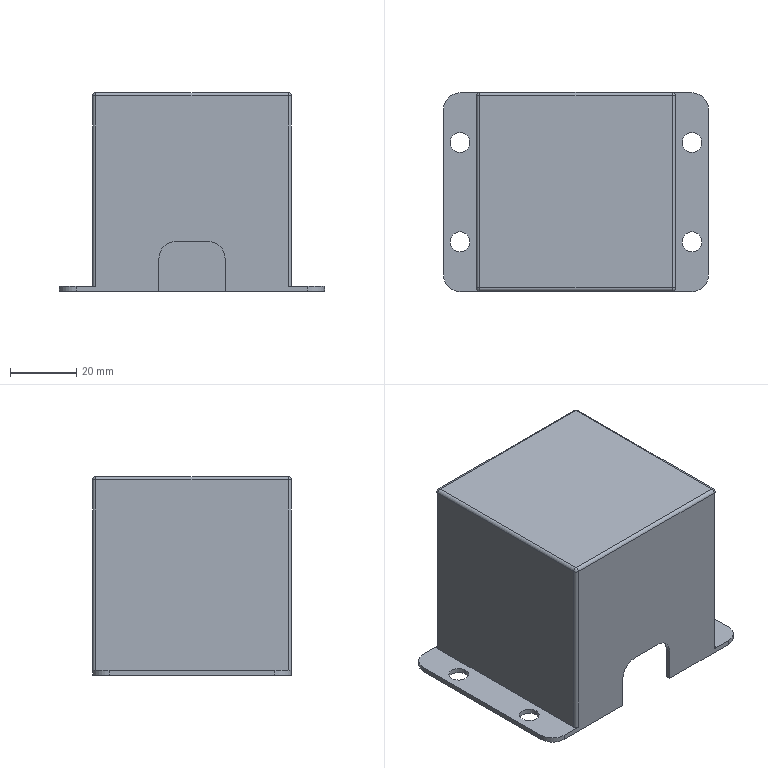Part | SolidWorks | features ICE 4, Fillet 3, Cut 1, Extrusion 1, MirrorPattern 1, Shell 1 | 1 solid | 46 faces | box 80 x 60 x 60 mm | volume 26373 mm3 | cylinder 24 | plane 18 | sphere 4 | commonest cylinder face diameters 2 x8 6 x8 10 x6 23 x2
STEP:
#1=CARTESIAN_POINT('',(-32.,15.,-30.));
#2=VERTEX_POINT('',#1);
#3=CARTESIAN_POINT('',(-38.,15.,-30.));
#4=VERTEX_POINT('',#3);
#5=CARTESIAN_POINT('',(-35.,15.,-30.));
#6=DIRECTION('',(0.,0.,-1.));
#7=DIRECTION('',(-1.,0.,0.));
#8=AXIS2_PLACEMENT_3D('',#5,#6,#7);
#9=CIRCLE('',#8,3.);
#10=EDGE_CURVE('',#2,#4,#9,.T.);
#11=ORIENTED_EDGE('',*,*,#10,.T.);
#12=CARTESIAN_POINT('',(-38.,15.,-28.5));
#13=VERTEX_POINT('',#12);
#14=CARTESIAN_POINT('',(-38.,15.,-30.));
#15=DIRECTION('',(0.,0.,1.));
#16=VECTOR('',#15,1000.);
#17=LINE('',#14,#16);
#18=EDGE_CURVE('',#4,#13,#17,.T.);
#19=ORIENTED_EDGE('',*,*,#18,.T.);
#20=CARTESIAN_POINT('',(-32.,15.,-28.5));
#21=VERTEX_POINT('',#20);
#22=CARTESIAN_POINT('',(-35.,15.,-28.5));
#23=DIRECTION('',(0.,0.,-1.));
#24=DIRECTION('',(-1.,0.,0.));
#25=AXIS2_PLACEMENT_3D('',#22,#23,#24);
#26=CIRCLE('',#25,3.);
#27=EDGE_CURVE('',#21,#13,#26,.T.);
#28=ORIENTED_EDGE('',*,*,#27,.F.);
#29=CARTESIAN_POINT('',(-32.,15.,-30.));
#30=DIRECTION('',(0.,0.,1.));
#31=VECTOR('',#30,1000.);
#32=LINE('',#29,#31);
#33=EDGE_CURVE('',#2,#21,#32,.T.);
#34=ORIENTED_EDGE('',*,*,#33,.F.);
#35=EDGE_LOOP('',(#11,#19,#28,#34));
#36=FACE_OUTER_BOUND('',#35,.T.);
#37=CARTESIAN_POINT('',(-35.,15.,-30.));
#38=DIRECTION('',(0.,0.,1.));
#39=DIRECTION('',(1.,0.,0.));
#40=AXIS2_PLACEMENT_3D('',#37,#38,#39);
#41=CYLINDRICAL_SURFACE('',#40,3.);
#42=ADVANCED_FACE('',(#36),#41,.F.);
#43=CARTESIAN_POINT('',(-32.,-15.,-30.));
#44=VERTEX_POINT('',#43);
#45=CARTESIAN_POINT('',(-38.,-15.,-30.));
#46=VERTEX_POINT('',#45);
#47=CARTESIAN_POINT('',(-35.,-15.,-30.));
#48=DIRECTION('',(0.,0.,-1.));
#49=DIRECTION('',(-1.,0.,0.));
#50=AXIS2_PLACEMENT_3D('',#47,#48,#49);
#51=CIRCLE('',#50,3.);
#52=EDGE_CURVE('',#44,#46,#51,.T.);
#53=ORIENTED_EDGE('',*,*,#52,.T.);
#54=CARTESIAN_POINT('',(-38.,-15.,-28.5));
#55=VERTEX_POINT('',#54);
#56=CARTESIAN_POINT('',(-38.,-15.,-30.));
#57=DIRECTION('',(0.,0.,1.));
#58=VECTOR('',#57,1000.);
#59=LINE('',#56,#58);
#60=EDGE_CURVE('',#46,#55,#59,.T.);
#61=ORIENTED_EDGE('',*,*,#60,.T.);
#62=CARTESIAN_POINT('',(-32.,-15.,-28.5));
#63=VERTEX_POINT('',#62);
#64=CARTESIAN_POINT('',(-35.,-15.,-28.5));
#65=DIRECTION('',(0.,0.,-1.));
#66=DIRECTION('',(-1.,0.,0.));
#67=AXIS2_PLACEMENT_3D('',#64,#65,#66);
#68=CIRCLE('',#67,3.);
#69=EDGE_CURVE('',#63,#55,#68,.T.);
#70=ORIENTED_EDGE('',*,*,#69,.F.);
#71=CARTESIAN_POINT('',(-32.,-15.,-30.));
#72=DIRECTION('',(0.,0.,1.));
#73=VECTOR('',#72,1000.);
#74=LINE('',#71,#73);
#75=EDGE_CURVE('',#44,#63,#74,.T.);
#76=ORIENTED_EDGE('',*,*,#75,.F.);
#77=EDGE_LOOP('',(#53,#61,#70,#76));
#78=FACE_OUTER_BOUND('',#77,.T.);
#79=CARTESIAN_POINT('',(-35.,-15.,-30.));
#80=DIRECTION('',(0.,0.,1.));
#81=DIRECTION('',(1.,0.,0.));
#82=AXIS2_PLACEMENT_3D('',#79,#80,#81);
#83=CYLINDRICAL_SURFACE('',#82,3.);
#84=ADVANCED_FACE('',(#78),#83,.F.);
#85=CARTESIAN_POINT('',(32.,15.,-30.));
#86=VERTEX_POINT('',#85);
#87=CARTESIAN_POINT('',(38.,15.,-30.));
#88=VERTEX_POINT('',#87);
#89=CARTESIAN_POINT('',(35.,15.,-30.));
#90=DIRECTION('',(0.,0.,1.));
#91=DIRECTION('',(1.,0.,0.));
#92=AXIS2_PLACEMENT_3D('',#89,#90,#91);
#93=CIRCLE('',#92,3.);
#94=EDGE_CURVE('',#86,#88,#93,.T.);
#95=ORIENTED_EDGE('',*,*,#94,.F.);
#96=CARTESIAN_POINT('',(32.,15.,-28.5));
#97=VERTEX_POINT('',#96);
#98=CARTESIAN_POINT('',(32.,15.,-30.));
#99=DIRECTION('',(0.,0.,1.));
#100=VECTOR('',#99,1000.);
#101=LINE('',#98,#100);
#102=EDGE_CURVE('',#86,#97,#101,.T.);
#103=ORIENTED_EDGE('',*,*,#102,.T.);
#104=CARTESIAN_POINT('',(38.,15.,-28.5));
#105=VERTEX_POINT('',#104);
#106=CARTESIAN_POINT('',(35.,15.,-28.5));
#107=DIRECTION('',(0.,0.,1.));
#108=DIRECTION('',(1.,0.,0.));
#109=AXIS2_PLACEMENT_3D('',#106,#107,#108);
#110=CIRCLE('',#109,3.);
#111=EDGE_CURVE('',#97,#105,#110,.T.);
#112=ORIENTED_EDGE('',*,*,#111,.T.);
#113=CARTESIAN_POINT('',(38.,15.,-30.));
#114=DIRECTION('',(0.,0.,1.));
#115=VECTOR('',#114,1000.);
#116=LINE('',#113,#115);
#117=EDGE_CURVE('',#88,#105,#116,.T.);
#118=ORIENTED_EDGE('',*,*,#117,.F.);
#119=EDGE_LOOP('',(#95,#103,#112,#118));
#120=FACE_OUTER_BOUND('',#119,.T.);
#121=CARTESIAN_POINT('',(35.,15.,-30.));
#122=DIRECTION('',(0.,0.,1.));
#123=DIRECTION('',(1.,0.,0.));
#124=AXIS2_PLACEMENT_3D('',#121,#122,#123);
#125=CYLINDRICAL_SURFACE('',#124,3.);
#126=ADVANCED_FACE('',(#120),#125,.F.);
#127=CARTESIAN_POINT('',(32.,-15.,-30.));
#128=VERTEX_POINT('',#127);
#129=CARTESIAN_POINT('',(38.,-15.,-30.));
#130=VERTEX_POINT('',#129);
#131=CARTESIAN_POINT('',(35.,-15.,-30.));
#132=DIRECTION('',(0.,0.,1.));
#133=DIRECTION('',(1.,0.,0.));
#134=AXIS2_PLACEMENT_3D('',#131,#132,#133);
#135=CIRCLE('',#134,3.);
#136=EDGE_CURVE('',#128,#130,#135,.T.);
#137=ORIENTED_EDGE('',*,*,#136,.F.);
#138=CARTESIAN_POINT('',(32.,-15.,-28.5));
#139=VERTEX_POINT('',#138);
#140=CARTESIAN_POINT('',(32.,-15.,-30.));
#141=DIRECTION('',(0.,0.,1.));
#142=VECTOR('',#141,1000.);
#143=LINE('',#140,#142);
#144=EDGE_CURVE('',#128,#139,#143,.T.);
#145=ORIENTED_EDGE('',*,*,#144,.T.);
#146=CARTESIAN_POINT('',(38.,-15.,-28.5));
#147=VERTEX_POINT('',#146);
#148=CARTESIAN_POINT('',(35.,-15.,-28.5));
#149=DIRECTION('',(0.,0.,1.));
#150=DIRECTION('',(1.,0.,0.));
#151=AXIS2_PLACEMENT_3D('',#148,#149,#150);
#152=CIRCLE('',#151,3.);
#153=EDGE_CURVE('',#139,#147,#152,.T.);
#154=ORIENTED_EDGE('',*,*,#153,.T.);
#155=CARTESIAN_POINT('',(38.,-15.,-30.));
#156=DIRECTION('',(0.,0.,1.));
#157=VECTOR('',#156,1000.);
#158=LINE('',#155,#157);
#159=EDGE_CURVE('',#130,#147,#158,.T.);
#160=ORIENTED_EDGE('',*,*,#159,.F.);
#161=EDGE_LOOP('',(#137,#145,#154,#160));
#162=FACE_OUTER_BOUND('',#161,.T.);
#163=CARTESIAN_POINT('',(35.,-15.,-30.));
#164=DIRECTION('',(0.,0.,1.));
#165=DIRECTION('',(1.,0.,0.));
#166=AXIS2_PLACEMENT_3D('',#163,#164,#165);
#167=CYLINDRICAL_SURFACE('',#166,3.);
#168=ADVANCED_FACE('',(#162),#167,.F.);
#169=CARTESIAN_POINT('',(0.,28.5,-11.5));
#170=VERTEX_POINT('',#169);
#171=CARTESIAN_POINT('',(0.,28.5,11.5));
#172=VERTEX_POINT('',#171);
#173=CARTESIAN_POINT('',(0.,28.5,0.));
#174=DIRECTION('',(0.,1.,0.));
#175=DIRECTION('',(0.,0.,-1.));
#176=AXIS2_PLACEMENT_3D('',#173,#174,#175);
#177=CIRCLE('',#176,11.5);
#178=EDGE_CURVE('',#170,#172,#177,.T.);
#179=ORIENTED_EDGE('',*,*,#178,.F.);
#180=CARTESIAN_POINT('',(0.,30.,-11.5));
#181=VERTEX_POINT('',#180);
#182=CARTESIAN_POINT('',(0.,-30.001,-11.5));
#183=DIRECTION('',(0.,1.,0.));
#184=VECTOR('',#183,1000.);
#185=LINE('',#182,#184);
#186=EDGE_CURVE('',#170,#181,#185,.T.);
#187=ORIENTED_EDGE('',*,*,#186,.T.);
#188=CARTESIAN_POINT('',(0.,30.,11.5));
#189=VERTEX_POINT('',#188);
#190=CARTESIAN_POINT('',(0.,30.,0.));
#191=DIRECTION('',(0.,1.,0.));
#192=DIRECTION('',(0.,0.,1.));
#193=AXIS2_PLACEMENT_3D('',#190,#191,#192);
#194=CIRCLE('',#193,11.5);
#195=EDGE_CURVE('',#181,#189,#194,.T.);
#196=ORIENTED_EDGE('',*,*,#195,.T.);
#197=CARTESIAN_POINT('',(0.,-30.001,11.5));
#198=DIRECTION('',(0.,1.,0.));
#199=VECTOR('',#198,1000.);
#200=LINE('',#197,#199);
#201=EDGE_CURVE('',#172,#189,#200,.T.);
#202=ORIENTED_EDGE('',*,*,#201,.F.);
#203=EDGE_LOOP('',(#179,#187,#196,#202));
#204=FACE_OUTER_BOUND('',#203,.T.);
#205=CARTESIAN_POINT('',(0.,-30.001,0.));
#206=DIRECTION('',(0.,1.,0.));
#207=DIRECTION('',(0.,0.,1.));
#208=AXIS2_PLACEMENT_3D('',#205,#206,#207);
#209=CYLINDRICAL_SURFACE('',#208,11.5);
#210=ADVANCED_FACE('',(#204),#209,.F.);
#211=CARTESIAN_POINT('',(-30.,-29.,29.));
#212=VERTEX_POINT('',#211);
#213=CARTESIAN_POINT('',(-30.,29.,29.));
#214=VERTEX_POINT('',#213);
#215=CARTESIAN_POINT('',(-30.,30.,29.));
#216=DIRECTION('',(0.,1.,0.));
#217=VECTOR('',#216,1000.);
#218=LINE('',#215,#217);
#219=EDGE_CURVE('',#212,#214,#218,.T.);
#220=ORIENTED_EDGE('',*,*,#219,.T.);
#221=CARTESIAN_POINT('',(-30.,29.,-28.5));
#222=VERTEX_POINT('',#221);
#223=CARTESIAN_POINT('',(-30.,29.,30.));
#224=DIRECTION('',(0.,0.,-1.));
#225=VECTOR('',#224,1000.);
#226=LINE('',#223,#225);
#227=EDGE_CURVE('',#214,#222,#226,.T.);
#228=ORIENTED_EDGE('',*,*,#227,.T.);
#229=CARTESIAN_POINT('',(-30.,-29.,-28.5));
#230=VERTEX_POINT('',#229);
#231=CARTESIAN_POINT('',(-30.,30.,-28.5));
#232=DIRECTION('',(0.,1.,0.));
#233=VECTOR('',#232,1000.);
#234=LINE('',#231,#233);
#235=EDGE_CURVE('',#230,#222,#234,.T.);
#236=ORIENTED_EDGE('',*,*,#235,.F.);
#237=CARTESIAN_POINT('',(-30.,-29.,30.));
#238=DIRECTION('',(0.,0.,1.));
#239=VECTOR('',#238,1000.);
#240=LINE('',#237,#239);
#241=EDGE_CURVE('',#230,#212,#240,.T.);
#242=ORIENTED_EDGE('',*,*,#241,.T.);
#243=EDGE_LOOP('',(#220,#228,#236,#242));
#244=FACE_OUTER_BOUND('',#243,.T.);
#245=CARTESIAN_POINT('',(-30.,30.,30.));
#246=DIRECTION('',(1.,0.,0.));
#247=DIRECTION('',(0.,1.,0.));
#248=AXIS2_PLACEMENT_3D('',#245,#246,#247);
#249=PLANE('',#248);
#250=ADVANCED_FACE('',(#244),#249,.F.);
#251=CARTESIAN_POINT('',(30.,29.,-28.5));
#252=VERTEX_POINT('',#251);
#253=CARTESIAN_POINT('',(30.,-29.,-28.5));
#254=VERTEX_POINT('',#253);
#255=CARTESIAN_POINT('',(30.,-30.,-28.5));
#256=DIRECTION('',(0.,-1.,0.));
#257=VECTOR('',#256,1000.);
#258=LINE('',#255,#257);
#259=EDGE_CURVE('',#252,#254,#258,.T.);
#260=ORIENTED_EDGE('',*,*,#259,.F.);
#261=CARTESIAN_POINT('',(30.,29.,29.));
#262=VERTEX_POINT('',#261);
#263=CARTESIAN_POINT('',(30.,29.,30.));
#264=DIRECTION('',(0.,0.,1.));
#265=VECTOR('',#264,1000.);
#266=LINE('',#263,#265);
#267=EDGE_CURVE('',#252,#262,#266,.T.);
#268=ORIENTED_EDGE('',*,*,#267,.T.);
#269=CARTESIAN_POINT('',(30.,-29.,29.));
#270=VERTEX_POINT('',#269);
#271=CARTESIAN_POINT('',(30.,-30.,29.));
#272=DIRECTION('',(0.,-1.,0.));
#273=VECTOR('',#272,1000.);
#274=LINE('',#271,#273);
#275=EDGE_CURVE('',#262,#270,#274,.T.);
#276=ORIENTED_EDGE('',*,*,#275,.T.);
#277=CARTESIAN_POINT('',(30.,-29.,30.));
#278=DIRECTION('',(0.,0.,-1.));
#279=VECTOR('',#278,1000.);
#280=LINE('',#277,#279);
#281=EDGE_CURVE('',#270,#254,#280,.T.);
#282=ORIENTED_EDGE('',*,*,#281,.T.);
#283=EDGE_LOOP('',(#260,#268,#276,#282));
#284=FACE_OUTER_BOUND('',#283,.T.);
#285=CARTESIAN_POINT('',(30.,30.,30.));
#286=DIRECTION('',(-1.,0.,0.));
#287=DIRECTION('',(0.,-1.,0.));
#288=AXIS2_PLACEMENT_3D('',#285,#286,#287);
#289=PLANE('',#288);
#290=ADVANCED_FACE('',(#284),#289,.F.);
#291=CARTESIAN_POINT('',(0.,30.,0.));
#292=DIRECTION('',(0.,1.,0.));
#293=DIRECTION('',(0.,0.,1.));
#294=AXIS2_PLACEMENT_3D('',#291,#292,#293);
#295=CIRCLE('',#294,11.5);
#296=EDGE_CURVE('',#189,#181,#295,.T.);
#297=ORIENTED_EDGE('',*,*,#296,.F.);
#298=ORIENTED_EDGE('',*,*,#195,.F.);
#299=EDGE_LOOP('',(#297,#298));
#300=FACE_BOUND('',#299,.T.);
#301=CARTESIAN_POINT('',(29.,30.,29.));
#302=VERTEX_POINT('',#301);
#303=CARTESIAN_POINT('',(29.,30.,-28.5));
#304=VERTEX_POINT('',#303);
#305=CARTESIAN_POINT('',(29.,30.,30.));
#306=DIRECTION('',(0.,0.,-1.));
#307=VECTOR('',#306,1000.);
#308=LINE('',#305,#307);
#309=EDGE_CURVE('',#302,#304,#308,.T.);
#310=ORIENTED_EDGE('',*,*,#309,.T.);
#311=CARTESIAN_POINT('',(35.,30.,-28.5));
#312=VERTEX_POINT('',#311);
#313=CARTESIAN_POINT('',(40.,30.,-28.5));
#314=DIRECTION('',(-1.,0.,0.));
#315=VECTOR('',#314,1000.);
#316=LINE('',#313,#315);
#317=EDGE_CURVE('',#312,#304,#316,.T.);
#318=ORIENTED_EDGE('',*,*,#317,.F.);
#319=CARTESIAN_POINT('',(35.,30.,-30.));
#320=VERTEX_POINT('',#319);
#321=CARTESIAN_POINT('',(35.,30.,-30.));
#322=DIRECTION('',(0.,0.,-1.));
#323=VECTOR('',#322,1000.);
#324=LINE('',#321,#323);
#325=EDGE_CURVE('',#312,#320,#324,.T.);
#326=ORIENTED_EDGE('',*,*,#325,.T.);
#327=CARTESIAN_POINT('',(-35.,30.,-30.));
#328=VERTEX_POINT('',#327);
#329=CARTESIAN_POINT('',(-30.,30.,-30.));
#330=DIRECTION('',(-1.,0.,0.));
#331=VECTOR('',#330,1000.);
#332=LINE('',#329,#331);
#333=EDGE_CURVE('',#320,#328,#332,.T.);
#334=ORIENTED_EDGE('',*,*,#333,.T.);
#335=CARTESIAN_POINT('',(-35.,30.,-28.5));
#336=VERTEX_POINT('',#335);
#337=CARTESIAN_POINT('',(-35.,30.,-28.5));
#338=DIRECTION('',(0.,0.,1.));
#339=VECTOR('',#338,1000.);
#340=LINE('',#337,#339);
#341=EDGE_CURVE('',#328,#336,#340,.T.);
#342=ORIENTED_EDGE('',*,*,#341,.T.);
#343=CARTESIAN_POINT('',(-29.,30.,-28.5));
#344=VERTEX_POINT('',#343);
#345=CARTESIAN_POINT('',(-40.,30.,-28.5));
#346=DIRECTION('',(1.,0.,0.));
#347=VECTOR('',#346,1000.);
#348=LINE('',#345,#347);
#349=EDGE_CURVE('',#336,#344,#348,.T.);
#350=ORIENTED_EDGE('',*,*,#349,.T.);
#351=CARTESIAN_POINT('',(-29.,30.,29.));
#352=VERTEX_POINT('',#351);
#353=CARTESIAN_POINT('',(-29.,30.,30.));
#354=DIRECTION('',(0.,0.,1.));
#355=VECTOR('',#354,1000.);
#356=LINE('',#353,#355);
#357=EDGE_CURVE('',#344,#352,#356,.T.);
#358=ORIENTED_EDGE('',*,*,#357,.T.);
#359=CARTESIAN_POINT('',(30.,30.,29.));
#360=DIRECTION('',(1.,0.,0.));
#361=VECTOR('',#360,1000.);
#362=LINE('',#359,#361);
#363=EDGE_CURVE('',#352,#302,#362,.T.);
#364=ORIENTED_EDGE('',*,*,#363,.T.);
#365=EDGE_LOOP('',(#310,#318,#326,#334,#342,#350,#358,#364));
#366=FACE_OUTER_BOUND('',#365,.T.);
#367=CARTESIAN_POINT('',(-30.,30.,30.));
#368=DIRECTION('',(0.,-1.,0.));
#369=DIRECTION('',(0.,0.,-1.));
#370=AXIS2_PLACEMENT_3D('',#367,#368,#369);
#371=PLANE('',#370);
#372=ADVANCED_FACE('',(#300,#366),#371,.F.);
#373=CARTESIAN_POINT('',(35.,-30.,-28.5));
#374=VERTEX_POINT('',#373);
#375=CARTESIAN_POINT('',(29.,-30.,-28.5));
#376=VERTEX_POINT('',#375);
#377=CARTESIAN_POINT('',(40.,-30.,-28.5));
#378=DIRECTION('',(-1.,0.,0.));
#379=VECTOR('',#378,1000.);
#380=LINE('',#377,#379);
#381=EDGE_CURVE('',#374,#376,#380,.T.);
#382=ORIENTED_EDGE('',*,*,#381,.T.);
#383=CARTESIAN_POINT('',(29.,-30.,29.));
#384=VERTEX_POINT('',#383);
#385=CARTESIAN_POINT('',(29.,-30.,30.));
#386=DIRECTION('',(0.,0.,1.));
#387=VECTOR('',#386,1000.);
#388=LINE('',#385,#387);
#389=EDGE_CURVE('',#376,#384,#388,.T.);
#390=ORIENTED_EDGE('',*,*,#389,.T.);
#391=CARTESIAN_POINT('',(-29.,-30.,29.));
#392=VERTEX_POINT('',#391);
#393=CARTESIAN_POINT('',(-30.,-30.,29.));
#394=DIRECTION('',(-1.,0.,0.));
#395=VECTOR('',#394,1000.);
#396=LINE('',#393,#395);
#397=EDGE_CURVE('',#384,#392,#396,.T.);
#398=ORIENTED_EDGE('',*,*,#397,.T.);
#399=CARTESIAN_POINT('',(-29.,-30.,-28.5));
#400=VERTEX_POINT('',#399);
#401=CARTESIAN_POINT('',(-29.,-30.,30.));
#402=DIRECTION('',(0.,0.,-1.));
#403=VECTOR('',#402,1000.);
#404=LINE('',#401,#403);
#405=EDGE_CURVE('',#392,#400,#404,.T.);
#406=ORIENTED_EDGE('',*,*,#405,.T.);
#407=CARTESIAN_POINT('',(-35.,-30.,-28.5));
#408=VERTEX_POINT('',#407);
#409=CARTESIAN_POINT('',(-40.,-30.,-28.5));
#410=DIRECTION('',(1.,0.,0.));
#411=VECTOR('',#410,1000.);
#412=LINE('',#409,#411);
#413=EDGE_CURVE('',#408,#400,#412,.T.);
#414=ORIENTED_EDGE('',*,*,#413,.F.);
#415=CARTESIAN_POINT('',(-35.,-30.,-30.));
#416=VERTEX_POINT('',#415);
#417=CARTESIAN_POINT('',(-35.,-30.,-30.));
#418=DIRECTION('',(0.,0.,-1.));
#419=VECTOR('',#418,1000.);
#420=LINE('',#417,#419);
#421=EDGE_CURVE('',#408,#416,#420,.T.);
#422=ORIENTED_EDGE('',*,*,#421,.T.);
#423=CARTESIAN_POINT('',(-10.,-30.,-30.));
#424=VERTEX_POINT('',#423);
#425=CARTESIAN_POINT('',(-30.,-30.,-30.));
#426=DIRECTION('',(1.,0.,0.));
#427=VECTOR('',#426,1000.);
#428=LINE('',#425,#427);
#429=EDGE_CURVE('',#416,#424,#428,.T.);
#430=ORIENTED_EDGE('',*,*,#429,.T.);
#431=CARTESIAN_POINT('',(-10.,-30.,-20.));
#432=VERTEX_POINT('',#431);
#433=CARTESIAN_POINT('',(-10.,-30.,-15.));
#434=DIRECTION('',(0.,0.,-1.));
#435=VECTOR('',#434,1000.);
#436=LINE('',#433,#435);
#437=EDGE_CURVE('',#432,#424,#436,.T.);
#438=ORIENTED_EDGE('',*,*,#437,.F.);
#439=CARTESIAN_POINT('',(-5.,-30.,-15.));
#440=VERTEX_POINT('',#439);
#441=CARTESIAN_POINT('',(-5.,-30.,-20.));
#442=DIRECTION('',(0.,1.,0.));
#443=DIRECTION('',(0.,0.,1.));
#444=AXIS2_PLACEMENT_3D('',#441,#442,#443);
#445=CIRCLE('',#444,5.);
#446=EDGE_CURVE('',#432,#440,#445,.T.);
#447=ORIENTED_EDGE('',*,*,#446,.T.);
#448=CARTESIAN_POINT('',(5.,-30.,-15.));
#449=VERTEX_POINT('',#448);
#450=CARTESIAN_POINT('',(-10.,-30.,-15.));
#451=DIRECTION('',(-1.,0.,0.));
#452=VECTOR('',#451,1000.);
#453=LINE('',#450,#452);
#454=EDGE_CURVE('',#449,#440,#453,.T.);
#455=ORIENTED_EDGE('',*,*,#454,.F.);
#456=CARTESIAN_POINT('',(10.,-30.,-20.));
#457=VERTEX_POINT('',#456);
#458=CARTESIAN_POINT('',(5.,-30.,-20.));
#459=DIRECTION('',(0.,1.,0.));
#460=DIRECTION('',(0.,0.,1.));
#461=AXIS2_PLACEMENT_3D('',#458,#459,#460);
#462=CIRCLE('',#461,5.);
#463=EDGE_CURVE('',#449,#457,#462,.T.);
#464=ORIENTED_EDGE('',*,*,#463,.T.);
#465=CARTESIAN_POINT('',(10.,-30.,-30.));
#466=VERTEX_POINT('',#465);
#467=CARTESIAN_POINT('',(10.,-30.,-15.));
#468=DIRECTION('',(0.,0.,1.));
#469=VECTOR('',#468,1000.);
#470=LINE('',#467,#469);
#471=EDGE_CURVE('',#466,#457,#470,.T.);
#472=ORIENTED_EDGE('',*,*,#471,.F.);
#473=CARTESIAN_POINT('',(35.,-30.,-30.));
#474=VERTEX_POINT('',#473);
#475=CARTESIAN_POINT('',(-30.,-30.,-30.));
#476=DIRECTION('',(1.,0.,0.));
#477=VECTOR('',#476,1000.);
#478=LINE('',#475,#477);
#479=EDGE_CURVE('',#466,#474,#478,.T.);
#480=ORIENTED_EDGE('',*,*,#479,.T.);
#481=CARTESIAN_POINT('',(35.,-30.,-28.5));
#482=DIRECTION('',(0.,0.,1.));
#483=VECTOR('',#482,1000.);
#484=LINE('',#481,#483);
#485=EDGE_CURVE('',#474,#374,#484,.T.);
#486=ORIENTED_EDGE('',*,*,#485,.T.);
#487=EDGE_LOOP('',(#382,#390,#398,#406,#414,#422,#430,#438,#447,#455,#464,#472,#480,#486));
#488=FACE_OUTER_BOUND('',#487,.T.);
#489=CARTESIAN_POINT('',(-30.,-30.,30.));
#490=DIRECTION('',(0.,1.,0.));
#491=DIRECTION('',(0.,0.,1.));
#492=AXIS2_PLACEMENT_3D('',#489,#490,#491);
#493=PLANE('',#492);
#494=ADVANCED_FACE('',(#488),#493,.F.);
#495=CARTESIAN_POINT('',(-29.,-29.,30.));
#496=VERTEX_POINT('',#495);
#497=CARTESIAN_POINT('',(29.,-29.,30.));
#498=VERTEX_POINT('',#497);
#499=CARTESIAN_POINT('',(30.,-29.,30.));
#500=DIRECTION('',(1.,0.,0.));
#501=VECTOR('',#500,1000.);
#502=LINE('',#499,#501);
#503=EDGE_CURVE('',#496,#498,#502,.T.);
#504=ORIENTED_EDGE('',*,*,#503,.T.);
#505=CARTESIAN_POINT('',(29.,29.,30.));
#506=VERTEX_POINT('',#505);
#507=CARTESIAN_POINT('',(29.,30.,30.));
#508=DIRECTION('',(0.,1.,0.));
#509=VECTOR('',#508,1000.);
#510=LINE('',#507,#509);
#511=EDGE_CURVE('',#498,#506,#510,.T.);
#512=ORIENTED_EDGE('',*,*,#511,.T.);
#513=CARTESIAN_POINT('',(-29.,29.,30.));
#514=VERTEX_POINT('',#513);
#515=CARTESIAN_POINT('',(-30.,29.,30.));
#516=DIRECTION('',(-1.,0.,0.));
#517=VECTOR('',#516,1000.);
#518=LINE('',#515,#517);
#519=EDGE_CURVE('',#506,#514,#518,.T.);
#520=ORIENTED_EDGE('',*,*,#519,.T.);
#521=CARTESIAN_POINT('',(-29.,-30.,30.));
#522=DIRECTION('',(0.,-1.,0.));
#523=VECTOR('',#522,1000.);
#524=LINE('',#521,#523);
#525=EDGE_CURVE('',#514,#496,#524,.T.);
#526=ORIENTED_EDGE('',*,*,#525,.T.);
#527=EDGE_LOOP('',(#504,#512,#520,#526));
#528=FACE_OUTER_BOUND('',#527,.T.);
#529=CARTESIAN_POINT('',(0.,0.,30.));
#530=DIRECTION('',(0.,0.,1.));
#531=DIRECTION('',(1.,0.,0.));
#532=AXIS2_PLACEMENT_3D('',#529,#530,#531);
#533=PLANE('',#532);
#534=ADVANCED_FACE('',(#528),#533,.T.);
#535=ORIENTED_EDGE('',*,*,#10,.F.);
#536=CARTESIAN_POINT('',(-35.,15.,-30.));
#537=DIRECTION('',(0.,0.,-1.));
#538=DIRECTION('',(-1.,0.,0.));
#539=AXIS2_PLACEMENT_3D('',#536,#537,#538);
#540=CIRCLE('',#539,3.);
#541=EDGE_CURVE('',#4,#2,#540,.T.);
#542=ORIENTED_EDGE('',*,*,#541,.F.);
#543=EDGE_LOOP('',(#535,#542));
#544=FACE_BOUND('',#543,.T.);
#545=ORIENTED_EDGE('',*,*,#52,.F.);
#546=CARTESIAN_POINT('',(-35.,-15.,-30.));
#547=DIRECTION('',(0.,0.,-1.));
#548=DIRECTION('',(-1.,0.,0.));
#549=AXIS2_PLACEMENT_3D('',#546,#547,#548);
#550=CIRCLE('',#549,3.);
#551=EDGE_CURVE('',#46,#44,#550,.T.);
#552=ORIENTED_EDGE('',*,*,#551,.F.);
#553=EDGE_LOOP('',(#545,#552));
#554=FACE_BOUND('',#553,.T.);
#555=CARTESIAN_POINT('',(35.,15.,-30.));
#556=DIRECTION('',(0.,0.,1.));
#557=DIRECTION('',(1.,0.,0.));
#558=AXIS2_PLACEMENT_3D('',#555,#556,#557);
#559=CIRCLE('',#558,3.);
#560=EDGE_CURVE('',#88,#86,#559,.T.);
#561=ORIENTED_EDGE('',*,*,#560,.T.);
#562=ORIENTED_EDGE('',*,*,#94,.T.);
#563=EDGE_LOOP('',(#561,#562));
#564=FACE_BOUND('',#563,.T.);
#565=CARTESIAN_POINT('',(35.,-15.,-30.));
#566=DIRECTION('',(0.,0.,1.));
#567=DIRECTION('',(1.,0.,0.));
#568=AXIS2_PLACEMENT_3D('',#565,#566,#567);
#569=CIRCLE('',#568,3.);
#570=EDGE_CURVE('',#130,#128,#569,.T.);
#571=ORIENTED_EDGE('',*,*,#570,.T.);
#572=ORIENTED_EDGE('',*,*,#136,.T.);
#573=EDGE_LOOP('',(#571,#572));
#574=FACE_BOUND('',#573,.T.);
#575=CARTESIAN_POINT('',(40.,-25.,-30.));
#576=VERTEX_POINT('',#575);
#577=CARTESIAN_POINT('',(40.,25.,-30.));
#578=VERTEX_POINT('',#577);
#579=CARTESIAN_POINT('',(40.,-30.,-30.));
#580=DIRECTION('',(0.,1.,0.));
#581=VECTOR('',#580,1000.);
#582=LINE('',#579,#581);
#583=EDGE_CURVE('',#576,#578,#582,.T.);
#584=ORIENTED_EDGE('',*,*,#583,.F.);
#585=CARTESIAN_POINT('',(35.,-25.,-30.));
#586=DIRECTION('',(0.,0.,-1.));
#587=DIRECTION('',(1.,0.,0.));
#588=AXIS2_PLACEMENT_3D('',#585,#586,#587);
#589=CIRCLE('',#588,5.);
#590=EDGE_CURVE('',#576,#474,#589,.T.);
#591=ORIENTED_EDGE('',*,*,#590,.T.);
#592=ORIENTED_EDGE('',*,*,#479,.F.);
#593=CARTESIAN_POINT('',(10.,-28.5,-30.));
#594=VERTEX_POINT('',#593);
#595=CARTESIAN_POINT('',(10.,30.001,-30.));
#596=DIRECTION('',(0.,-1.,0.));
#597=VECTOR('',#596,1000.);
#598=LINE('',#595,#597);
#599=EDGE_CURVE('',#594,#466,#598,.T.);
#600=ORIENTED_EDGE('',*,*,#599,.F.);
#601=CARTESIAN_POINT('',(28.5,-28.5,-30.));
#602=VERTEX_POINT('',#601);
#603=CARTESIAN_POINT('',(-30.,-28.5,-30.));
#604=DIRECTION('',(1.,0.,0.));
#605=VECTOR('',#604,1000.);
#606=LINE('',#603,#605);
#607=EDGE_CURVE('',#594,#602,#606,.T.);
#608=ORIENTED_EDGE('',*,*,#607,.T.);
#609=CARTESIAN_POINT('',(28.5,28.5,-30.));
#610=VERTEX_POINT('',#609);
#611=CARTESIAN_POINT('',(28.5,30.,-30.));
#612=DIRECTION('',(0.,1.,0.));
#613=VECTOR('',#612,1000.);
#614=LINE('',#611,#613);
#615=EDGE_CURVE('',#602,#610,#614,.T.);
#616=ORIENTED_EDGE('',*,*,#615,.T.);
#617=CARTESIAN_POINT('',(-28.5,28.5,-30.));
#618=VERTEX_POINT('',#617);
#619=CARTESIAN_POINT('',(-30.,28.5,-30.));
#620=DIRECTION('',(-1.,0.,0.));
#621=VECTOR('',#620,1000.);
#622=LINE('',#619,#621);
#623=EDGE_CURVE('',#610,#618,#622,.T.);
#624=ORIENTED_EDGE('',*,*,#623,.T.);
#625=CARTESIAN_POINT('',(-28.5,-28.5,-30.));
#626=VERTEX_POINT('',#625);
#627=CARTESIAN_POINT('',(-28.5,30.,-30.));
#628=DIRECTION('',(0.,-1.,0.));
#629=VECTOR('',#628,1000.);
#630=LINE('',#627,#629);
#631=EDGE_CURVE('',#618,#626,#630,.T.);
#632=ORIENTED_EDGE('',*,*,#631,.T.);
#633=CARTESIAN_POINT('',(-10.,-28.5,-30.));
#634=VERTEX_POINT('',#633);
#635=CARTESIAN_POINT('',(-30.,-28.5,-30.));
#636=DIRECTION('',(1.,0.,0.));
#637=VECTOR('',#636,1000.);
#638=LINE('',#635,#637);
#639=EDGE_CURVE('',#626,#634,#638,.T.);
#640=ORIENTED_EDGE('',*,*,#639,.T.);
#641=CARTESIAN_POINT('',(-10.,30.001,-30.));
#642=DIRECTION('',(0.,-1.,0.));
#643=VECTOR('',#642,1000.);
#644=LINE('',#641,#643);
#645=EDGE_CURVE('',#634,#424,#644,.T.);
#646=ORIENTED_EDGE('',*,*,#645,.T.);
#647=ORIENTED_EDGE('',*,*,#429,.F.);
#648=CARTESIAN_POINT('',(-40.,-25.,-30.));
#649=VERTEX_POINT('',#648);
#650=CARTESIAN_POINT('',(-35.,-25.,-30.));
#651=DIRECTION('',(0.,0.,-1.));
#652=DIRECTION('',(1.,0.,0.));
#653=AXIS2_PLACEMENT_3D('',#650,#651,#652);
#654=CIRCLE('',#653,5.);
#655=EDGE_CURVE('',#416,#649,#654,.T.);
#656=ORIENTED_EDGE('',*,*,#655,.T.);
#657=CARTESIAN_POINT('',(-40.,25.,-30.));
#658=VERTEX_POINT('',#657);
#659=CARTESIAN_POINT('',(-40.,30.,-30.));
#660=DIRECTION('',(0.,-1.,0.));
#661=VECTOR('',#660,1000.);
#662=LINE('',#659,#661);
#663=EDGE_CURVE('',#658,#649,#662,.T.);
#664=ORIENTED_EDGE('',*,*,#663,.F.);
#665=CARTESIAN_POINT('',(-35.,25.,-30.));
#666=DIRECTION('',(0.,0.,-1.));
#667=DIRECTION('',(1.,0.,0.));
#668=AXIS2_PLACEMENT_3D('',#665,#666,#667);
#669=CIRCLE('',#668,5.);
#670=EDGE_CURVE('',#658,#328,#669,.T.);
#671=ORIENTED_EDGE('',*,*,#670,.T.);
#672=ORIENTED_EDGE('',*,*,#333,.F.);
#673=CARTESIAN_POINT('',(35.,25.,-30.));
#674=DIRECTION('',(0.,0.,-1.));
#675=DIRECTION('',(1.,0.,0.));
#676=AXIS2_PLACEMENT_3D('',#673,#674,#675);
#677=CIRCLE('',#676,5.);
#678=EDGE_CURVE('',#320,#578,#677,.T.);
#679=ORIENTED_EDGE('',*,*,#678,.T.);
#680=EDGE_LOOP('',(#584,#591,#592,#600,#608,#616,#624,#632,#640,#646,#647,#656,#664,#671,#672,#679));
#681=FACE_OUTER_BOUND('',#680,.T.);
#682=CARTESIAN_POINT('',(0.,0.,-30.));
#683=DIRECTION('',(0.,0.,1.));
#684=DIRECTION('',(1.,0.,0.));
#685=AXIS2_PLACEMENT_3D('',#682,#683,#684);
#686=PLANE('',#685);
#687=ADVANCED_FACE('',(#544,#554,#564,#574,#681),#686,.F.);
#688=ORIENTED_EDGE('',*,*,#615,.F.);
#689=CARTESIAN_POINT('',(28.5,-28.5,28.5));
#690=VERTEX_POINT('',#689);
#691=CARTESIAN_POINT('',(28.5,-28.5,30.));
#692=DIRECTION('',(0.,0.,-1.));
#693=VECTOR('',#692,1000.);
#694=LINE('',#691,#693);
#695=EDGE_CURVE('',#690,#602,#694,.T.);
#696=ORIENTED_EDGE('',*,*,#695,.F.);
#697=CARTESIAN_POINT('',(28.5,28.5,28.5));
#698=VERTEX_POINT('',#697);
#699=CARTESIAN_POINT('',(28.5,30.,28.5));
#700=DIRECTION('',(0.,1.,0.));
#701=VECTOR('',#700,1000.);
#702=LINE('',#699,#701);
#703=EDGE_CURVE('',#690,#698,#702,.T.);
#704=ORIENTED_EDGE('',*,*,#703,.T.);
#705=CARTESIAN_POINT('',(28.5,28.5,30.));
#706=DIRECTION('',(0.,0.,-1.));
#707=VECTOR('',#706,1000.);
#708=LINE('',#705,#707);
#709=EDGE_CURVE('',#698,#610,#708,.T.);
#710=ORIENTED_EDGE('',*,*,#709,.T.);
#711=EDGE_LOOP('',(#688,#696,#704,#710));
#712=FACE_OUTER_BOUND('',#711,.T.);
#713=CARTESIAN_POINT('',(28.5,30.,30.));
#714=DIRECTION('',(-1.,0.,0.));
#715=DIRECTION('',(0.,-1.,0.));
#716=AXIS2_PLACEMENT_3D('',#713,#714,#715);
#717=PLANE('',#716);
#718=ADVANCED_FACE('',(#712),#717,.T.);
#719=CARTESIAN_POINT('',(0.,28.5,0.));
#720=DIRECTION('',(0.,1.,0.));
#721=DIRECTION('',(0.,0.,-1.));
#722=AXIS2_PLACEMENT_3D('',#719,#720,#721);
#723=CIRCLE('',#722,11.5);
#724=EDGE_CURVE('',#172,#170,#723,.T.);
#725=ORIENTED_EDGE('',*,*,#724,.T.);
#726=ORIENTED_EDGE('',*,*,#178,.T.);
#727=EDGE_LOOP('',(#725,#726));
#728=FACE_BOUND('',#727,.T.);
#729=ORIENTED_EDGE('',*,*,#623,.F.);
#730=ORIENTED_EDGE('',*,*,#709,.F.);
#731=CARTESIAN_POINT('',(-28.5,28.5,28.5));
#732=VERTEX_POINT('',#731);
#733=CARTESIAN_POINT('',(-30.,28.5,28.5));
#734=DIRECTION('',(-1.,0.,0.));
#735=VECTOR('',#734,1000.);
#736=LINE('',#733,#735);
#737=EDGE_CURVE('',#698,#732,#736,.T.);
#738=ORIENTED_EDGE('',*,*,#737,.T.);
#739=CARTESIAN_POINT('',(-28.5,28.5,30.));
#740=DIRECTION('',(0.,0.,-1.));
#741=VECTOR('',#740,1000.);
#742=LINE('',#739,#741);
#743=EDGE_CURVE('',#732,#618,#742,.T.);
#744=ORIENTED_EDGE('',*,*,#743,.T.);
#745=EDGE_LOOP('',(#729,#730,#738,#744));
#746=FACE_OUTER_BOUND('',#745,.T.);
#747=CARTESIAN_POINT('',(-30.,28.5,30.));
#748=DIRECTION('',(0.,-1.,0.));
#749=DIRECTION('',(0.,0.,-1.));
#750=AXIS2_PLACEMENT_3D('',#747,#748,#749);
#751=PLANE('',#750);
#752=ADVANCED_FACE('',(#728,#746),#751,.T.);
#753=ORIENTED_EDGE('',*,*,#631,.F.);
#754=ORIENTED_EDGE('',*,*,#743,.F.);
#755=CARTESIAN_POINT('',(-28.5,-28.5,28.5));
#756=VERTEX_POINT('',#755);
#757=CARTESIAN_POINT('',(-28.5,30.,28.5));
#758=DIRECTION('',(0.,-1.,0.));
#759=VECTOR('',#758,1000.);
#760=LINE('',#757,#759);
#761=EDGE_CURVE('',#732,#756,#760,.T.);
#762=ORIENTED_EDGE('',*,*,#761,.T.);
#763=CARTESIAN_POINT('',(-28.5,-28.5,30.));
#764=DIRECTION('',(0.,0.,-1.));
#765=VECTOR('',#764,1000.);
#766=LINE('',#763,#765);
#767=EDGE_CURVE('',#756,#626,#766,.T.);
#768=ORIENTED_EDGE('',*,*,#767,.T.);
#769=EDGE_LOOP('',(#753,#754,#762,#768));
#770=FACE_OUTER_BOUND('',#769,.T.);
#771=CARTESIAN_POINT('',(-28.5,30.,30.));
#772=DIRECTION('',(1.,0.,0.));
#773=DIRECTION('',(0.,1.,0.));
#774=AXIS2_PLACEMENT_3D('',#771,#772,#773);
#775=PLANE('',#774);
#776=ADVANCED_FACE('',(#770),#775,.T.);
#777=CARTESIAN_POINT('',(10.,-28.5,-20.));
#778=VERTEX_POINT('',#777);
#779=CARTESIAN_POINT('',(10.,-28.5,-15.));
#780=DIRECTION('',(0.,0.,1.));
#781=VECTOR('',#780,1000.);
#782=LINE('',#779,#781);
#783=EDGE_CURVE('',#594,#778,#782,.T.);
#784=ORIENTED_EDGE('',*,*,#783,.T.);
#785=CARTESIAN_POINT('',(5.,-28.5,-15.));
#786=VERTEX_POINT('',#785);
#787=CARTESIAN_POINT('',(5.,-28.5,-20.));
#788=DIRECTION('',(0.,-1.,0.));
#789=DIRECTION('',(0.,0.,1.));
#790=AXIS2_PLACEMENT_3D('',#787,#788,#789);
#791=CIRCLE('',#790,5.);
#792=EDGE_CURVE('',#778,#786,#791,.T.);
#793=ORIENTED_EDGE('',*,*,#792,.T.);
#794=CARTESIAN_POINT('',(-5.,-28.5,-15.));
#795=VERTEX_POINT('',#794);
#796=CARTESIAN_POINT('',(-10.,-28.5,-15.));
#797=DIRECTION('',(-1.,0.,0.));
#798=VECTOR('',#797,1000.);
#799=LINE('',#796,#798);
#800=EDGE_CURVE('',#786,#795,#799,.T.);
#801=ORIENTED_EDGE('',*,*,#800,.T.);
#802=CARTESIAN_POINT('',(-10.,-28.5,-20.));
#803=VERTEX_POINT('',#802);
#804=CARTESIAN_POINT('',(-5.,-28.5,-20.));
#805=DIRECTION('',(0.,-1.,0.));
#806=DIRECTION('',(0.,0.,1.));
#807=AXIS2_PLACEMENT_3D('',#804,#805,#806);
#808=CIRCLE('',#807,5.);
#809=EDGE_CURVE('',#795,#803,#808,.T.);
#810=ORIENTED_EDGE('',*,*,#809,.T.);
#811=CARTESIAN_POINT('',(-10.,-28.5,-15.));
#812=DIRECTION('',(0.,0.,-1.));
#813=VECTOR('',#812,1000.);
#814=LINE('',#811,#813);
#815=EDGE_CURVE('',#803,#634,#814,.T.);
#816=ORIENTED_EDGE('',*,*,#815,.T.);
#817=ORIENTED_EDGE('',*,*,#639,.F.);
#818=ORIENTED_EDGE('',*,*,#767,.F.);
#819=CARTESIAN_POINT('',(-30.,-28.5,28.5));
#820=DIRECTION('',(1.,0.,0.));
#821=VECTOR('',#820,1000.);
#822=LINE('',#819,#821);
#823=EDGE_CURVE('',#756,#690,#822,.T.);
#824=ORIENTED_EDGE('',*,*,#823,.T.);
#825=ORIENTED_EDGE('',*,*,#695,.T.);
#826=ORIENTED_EDGE('',*,*,#607,.F.);
#827=EDGE_LOOP('',(#784,#793,#801,#810,#816,#817,#818,#824,#825,#826));
#828=FACE_OUTER_BOUND('',#827,.T.);
#829=CARTESIAN_POINT('',(-30.,-28.5,30.));
#830=DIRECTION('',(0.,1.,0.));
#831=DIRECTION('',(0.,0.,1.));
#832=AXIS2_PLACEMENT_3D('',#829,#830,#831);
#833=PLANE('',#832);
#834=ADVANCED_FACE('',(#828),#833,.T.);
#835=ORIENTED_EDGE('',*,*,#703,.F.);
#836=ORIENTED_EDGE('',*,*,#823,.F.);
#837=ORIENTED_EDGE('',*,*,#761,.F.);
#838=ORIENTED_EDGE('',*,*,#737,.F.);
#839=EDGE_LOOP('',(#835,#836,#837,#838));
#840=FACE_OUTER_BOUND('',#839,.T.);
#841=CARTESIAN_POINT('',(0.,0.,28.5));
#842=DIRECTION('',(0.,0.,1.));
#843=DIRECTION('',(1.,0.,0.));
#844=AXIS2_PLACEMENT_3D('',#841,#842,#843);
#845=PLANE('',#844);
#846=ADVANCED_FACE('',(#840),#845,.F.);
#847=CARTESIAN_POINT('',(35.,15.,-28.5));
#848=DIRECTION('',(0.,0.,1.));
#849=DIRECTION('',(1.,0.,0.));
#850=AXIS2_PLACEMENT_3D('',#847,#848,#849);
#851=CIRCLE('',#850,3.);
#852=EDGE_CURVE('',#105,#97,#851,.T.);
#853=ORIENTED_EDGE('',*,*,#852,.F.);
#854=ORIENTED_EDGE('',*,*,#111,.F.);
#855=EDGE_LOOP('',(#853,#854));
#856=FACE_BOUND('',#855,.T.);
#857=CARTESIAN_POINT('',(35.,-15.,-28.5));
#858=DIRECTION('',(0.,0.,1.));
#859=DIRECTION('',(1.,0.,0.));
#860=AXIS2_PLACEMENT_3D('',#857,#858,#859);
#861=CIRCLE('',#860,3.);
#862=EDGE_CURVE('',#147,#139,#861,.T.);
#863=ORIENTED_EDGE('',*,*,#862,.F.);
#864=ORIENTED_EDGE('',*,*,#153,.F.);
#865=EDGE_LOOP('',(#863,#864));
#866=FACE_BOUND('',#865,.T.);
#867=ORIENTED_EDGE('',*,*,#381,.F.);
#868=CARTESIAN_POINT('',(40.,-25.,-28.5));
#869=VERTEX_POINT('',#868);
#870=CARTESIAN_POINT('',(35.,-25.,-28.5));
#871=DIRECTION('',(0.,0.,1.));
#872=DIRECTION('',(-1.,0.,0.));
#873=AXIS2_PLACEMENT_3D('',#870,#871,#872);
#874=CIRCLE('',#873,5.);
#875=EDGE_CURVE('',#374,#869,#874,.T.);
#876=ORIENTED_EDGE('',*,*,#875,.T.);
#877=CARTESIAN_POINT('',(40.,25.,-28.5));
#878=VERTEX_POINT('',#877);
#879=CARTESIAN_POINT('',(40.,-30.,-28.5));
#880=DIRECTION('',(0.,-1.,0.));
#881=VECTOR('',#880,1000.);
#882=LINE('',#879,#881);
#883=EDGE_CURVE('',#878,#869,#882,.T.);
#884=ORIENTED_EDGE('',*,*,#883,.F.);
#885=CARTESIAN_POINT('',(35.,25.,-28.5));
#886=DIRECTION('',(0.,0.,1.));
#887=DIRECTION('',(-1.,0.,0.));
#888=AXIS2_PLACEMENT_3D('',#885,#886,#887);
#889=CIRCLE('',#888,5.);
#890=EDGE_CURVE('',#878,#312,#889,.T.);
#891=ORIENTED_EDGE('',*,*,#890,.T.);
#892=ORIENTED_EDGE('',*,*,#317,.T.);
#893=CARTESIAN_POINT('',(29.,29.,-28.5));
#894=DIRECTION('',(0.,0.,-1.));
#895=DIRECTION('',(-1.,0.,0.));
#896=AXIS2_PLACEMENT_3D('',#893,#894,#895);
#897=CIRCLE('',#896,1.);
#898=EDGE_CURVE('',#304,#252,#897,.T.);
#899=ORIENTED_EDGE('',*,*,#898,.T.);
#900=ORIENTED_EDGE('',*,*,#259,.T.);
#901=CARTESIAN_POINT('',(29.,-29.,-28.5));
#902=DIRECTION('',(0.,0.,-1.));
#903=DIRECTION('',(-1.,0.,0.));
#904=AXIS2_PLACEMENT_3D('',#901,#902,#903);
#905=CIRCLE('',#904,1.);
#906=EDGE_CURVE('',#254,#376,#905,.T.);
#907=ORIENTED_EDGE('',*,*,#906,.T.);
#908=EDGE_LOOP('',(#867,#876,#884,#891,#892,#899,#900,#907));
#909=FACE_OUTER_BOUND('',#908,.T.);
#910=CARTESIAN_POINT('',(40.,-30.,-28.5));
#911=DIRECTION('',(0.,0.,-1.));
#912=DIRECTION('',(-1.,0.,0.));
#913=AXIS2_PLACEMENT_3D('',#910,#911,#912);
#914=PLANE('',#913);
#915=ADVANCED_FACE('',(#856,#866,#909),#914,.F.);
#916=ORIENTED_EDGE('',*,*,#883,.T.);
#917=CARTESIAN_POINT('',(40.,-25.,-30.));
#918=DIRECTION('',(0.,0.,-1.));
#919=VECTOR('',#918,1000.);
#920=LINE('',#917,#919);
#921=EDGE_CURVE('',#869,#576,#920,.T.);
#922=ORIENTED_EDGE('',*,*,#921,.T.);
#923=ORIENTED_EDGE('',*,*,#583,.T.);
#924=CARTESIAN_POINT('',(40.,25.,-28.5));
#925=DIRECTION('',(0.,0.,1.));
#926=VECTOR('',#925,1000.);
#927=LINE('',#924,#926);
#928=EDGE_CURVE('',#578,#878,#927,.T.);
#929=ORIENTED_EDGE('',*,*,#928,.T.);
#930=EDGE_LOOP('',(#916,#922,#923,#929));
#931=FACE_OUTER_BOUND('',#930,.T.);
#932=CARTESIAN_POINT('',(40.,0.,0.));
#933=DIRECTION('',(1.,0.,0.));
#934=DIRECTION('',(0.,1.,0.));
#935=AXIS2_PLACEMENT_3D('',#932,#933,#934);
#936=PLANE('',#935);
#937=ADVANCED_FACE('',(#931),#936,.T.);
#938=ORIENTED_EDGE('',*,*,#27,.T.);
#939=CARTESIAN_POINT('',(-35.,15.,-28.5));
#940=DIRECTION('',(0.,0.,-1.));
#941=DIRECTION('',(-1.,0.,0.));
#942=AXIS2_PLACEMENT_3D('',#939,#940,#941);
#943=CIRCLE('',#942,3.);
#944=EDGE_CURVE('',#13,#21,#943,.T.);
#945=ORIENTED_EDGE('',*,*,#944,.T.);
#946=EDGE_LOOP('',(#938,#945));
#947=FACE_BOUND('',#946,.T.);
#948=ORIENTED_EDGE('',*,*,#69,.T.);
#949=CARTESIAN_POINT('',(-35.,-15.,-28.5));
#950=DIRECTION('',(0.,0.,-1.));
#951=DIRECTION('',(-1.,0.,0.));
#952=AXIS2_PLACEMENT_3D('',#949,#950,#951);
#953=CIRCLE('',#952,3.);
#954=EDGE_CURVE('',#55,#63,#953,.T.);
#955=ORIENTED_EDGE('',*,*,#954,.T.);
#956=EDGE_LOOP('',(#948,#955));
#957=FACE_BOUND('',#956,.T.);
#958=CARTESIAN_POINT('',(-40.,-25.,-28.5));
#959=VERTEX_POINT('',#958);
#960=CARTESIAN_POINT('',(-40.,25.,-28.5));
#961=VERTEX_POINT('',#960);
#962=CARTESIAN_POINT('',(-40.,30.,-28.5));
#963=DIRECTION('',(0.,1.,0.));
#964=VECTOR('',#963,1000.);
#965=LINE('',#962,#964);
#966=EDGE_CURVE('',#959,#961,#965,.T.);
#967=ORIENTED_EDGE('',*,*,#966,.F.);
#968=CARTESIAN_POINT('',(-35.,-25.,-28.5));
#969=DIRECTION('',(0.,0.,1.));
#970=DIRECTION('',(0.,1.,0.));
#971=AXIS2_PLACEMENT_3D('',#968,#969,#970);
#972=CIRCLE('',#971,5.);
#973=EDGE_CURVE('',#959,#408,#972,.T.);
#974=ORIENTED_EDGE('',*,*,#973,.T.);
#975=ORIENTED_EDGE('',*,*,#413,.T.);
#976=CARTESIAN_POINT('',(-29.,-29.,-28.5));
#977=DIRECTION('',(0.,0.,-1.));
#978=DIRECTION('',(0.,1.,0.));
#979=AXIS2_PLACEMENT_3D('',#976,#977,#978);
#980=CIRCLE('',#979,1.);
#981=EDGE_CURVE('',#400,#230,#980,.T.);
#982=ORIENTED_EDGE('',*,*,#981,.T.);
#983=ORIENTED_EDGE('',*,*,#235,.T.);
#984=CARTESIAN_POINT('',(-29.,29.,-28.5));
#985=DIRECTION('',(0.,0.,-1.));
#986=DIRECTION('',(0.,1.,0.));
#987=AXIS2_PLACEMENT_3D('',#984,#985,#986);
#988=CIRCLE('',#987,1.);
#989=EDGE_CURVE('',#222,#344,#988,.T.);
#990=ORIENTED_EDGE('',*,*,#989,.T.);
#991=ORIENTED_EDGE('',*,*,#349,.F.);
#992=CARTESIAN_POINT('',(-35.,25.,-28.5));
#993=DIRECTION('',(0.,0.,1.));
#994=DIRECTION('',(0.,1.,0.));
#995=AXIS2_PLACEMENT_3D('',#992,#993,#994);
#996=CIRCLE('',#995,5.);
#997=EDGE_CURVE('',#336,#961,#996,.T.);
#998=ORIENTED_EDGE('',*,*,#997,.T.);
#999=EDGE_LOOP('',(#967,#974,#975,#982,#983,#990,#991,#998));
#1000=FACE_OUTER_BOUND('',#999,.T.);
#1001=CARTESIAN_POINT('',(-40.,30.,-28.5));
#1002=DIRECTION('',(0.,0.,-1.));
#1003=DIRECTION('',(0.,1.,0.));
#1004=AXIS2_PLACEMENT_3D('',#1001,#1002,#1003);
#1005=PLANE('',#1004);
#1006=ADVANCED_FACE('',(#947,#957,#1000),#1005,.F.);
#1007=ORIENTED_EDGE('',*,*,#663,.T.);
#1008=CARTESIAN_POINT('',(-40.,-25.,-28.5));
#1009=DIRECTION('',(0.,0.,1.));
#1010=VECTOR('',#1009,1000.);
#1011=LINE('',#1008,#1010);
#1012=EDGE_CURVE('',#649,#959,#1011,.T.);
#1013=ORIENTED_EDGE('',*,*,#1012,.T.);
#1014=ORIENTED_EDGE('',*,*,#966,.T.);
#1015=CARTESIAN_POINT('',(-40.,25.,-30.));
#1016=DIRECTION('',(0.,0.,-1.));
#1017=VECTOR('',#1016,1000.);
#1018=LINE('',#1015,#1017);
#1019=EDGE_CURVE('',#961,#658,#1018,.T.);
#1020=ORIENTED_EDGE('',*,*,#1019,.T.);
#1021=EDGE_LOOP('',(#1007,#1013,#1014,#1020));
#1022=FACE_OUTER_BOUND('',#1021,.T.);
#1023=CARTESIAN_POINT('',(-40.,0.,0.));
#1024=DIRECTION('',(-1.,0.,0.));
#1025=DIRECTION('',(0.,-1.,0.));
#1026=AXIS2_PLACEMENT_3D('',#1023,#1024,#1025);
#1027=PLANE('',#1026);
#1028=ADVANCED_FACE('',(#1022),#1027,.T.);
#1029=ORIENTED_EDGE('',*,*,#471,.T.);
#1030=CARTESIAN_POINT('',(10.,-28.5,-20.));
#1031=DIRECTION('',(0.,1.,0.));
#1032=VECTOR('',#1031,1000.);
#1033=LINE('',#1030,#1032);
#1034=EDGE_CURVE('',#457,#778,#1033,.T.);
#1035=ORIENTED_EDGE('',*,*,#1034,.T.);
#1036=ORIENTED_EDGE('',*,*,#783,.F.);
#1037=ORIENTED_EDGE('',*,*,#599,.T.);
#1038=EDGE_LOOP('',(#1029,#1035,#1036,#1037));
#1039=FACE_OUTER_BOUND('',#1038,.T.);
#1040=CARTESIAN_POINT('',(10.,30.001,-15.));
#1041=DIRECTION('',(1.,0.,0.));
#1042=DIRECTION('',(0.,0.,-1.));
#1043=AXIS2_PLACEMENT_3D('',#1040,#1041,#1042);
#1044=PLANE('',#1043);
#1045=ADVANCED_FACE('',(#1039),#1044,.F.);
#1046=ORIENTED_EDGE('',*,*,#800,.F.);
#1047=CARTESIAN_POINT('',(5.,-30.,-15.));
#1048=DIRECTION('',(0.,-1.,0.));
#1049=VECTOR('',#1048,1000.);
#1050=LINE('',#1047,#1049);
#1051=EDGE_CURVE('',#786,#449,#1050,.T.);
#1052=ORIENTED_EDGE('',*,*,#1051,.T.);
#1053=ORIENTED_EDGE('',*,*,#454,.T.);
#1054=CARTESIAN_POINT('',(-5.,-28.5,-15.));
#1055=DIRECTION('',(0.,1.,0.));
#1056=VECTOR('',#1055,1000.);
#1057=LINE('',#1054,#1056);
#1058=EDGE_CURVE('',#440,#795,#1057,.T.);
#1059=ORIENTED_EDGE('',*,*,#1058,.T.);
#1060=EDGE_LOOP('',(#1046,#1052,#1053,#1059));
#1061=FACE_OUTER_BOUND('',#1060,.T.);
#1062=CARTESIAN_POINT('',(-10.,30.001,-15.));
#1063=DIRECTION('',(0.,0.,1.));
#1064=DIRECTION('',(1.,0.,0.));
#1065=AXIS2_PLACEMENT_3D('',#1062,#1063,#1064);
#1066=PLANE('',#1065);
#1067=ADVANCED_FACE('',(#1061),#1066,.F.);
#1068=ORIENTED_EDGE('',*,*,#815,.F.);
#1069=CARTESIAN_POINT('',(-10.,-30.,-20.));
#1070=DIRECTION('',(0.,-1.,0.));
#1071=VECTOR('',#1070,1000.);
#1072=LINE('',#1069,#1071);
#1073=EDGE_CURVE('',#803,#432,#1072,.T.);
#1074=ORIENTED_EDGE('',*,*,#1073,.T.);
#1075=ORIENTED_EDGE('',*,*,#437,.T.);
#1076=ORIENTED_EDGE('',*,*,#645,.F.);
#1077=EDGE_LOOP('',(#1068,#1074,#1075,#1076));
#1078=FACE_OUTER_BOUND('',#1077,.T.);
#1079=CARTESIAN_POINT('',(-10.,30.001,-15.));
#1080=DIRECTION('',(-1.,0.,0.));
#1081=DIRECTION('',(0.,0.,1.));
#1082=AXIS2_PLACEMENT_3D('',#1079,#1080,#1081);
#1083=PLANE('',#1082);
#1084=ADVANCED_FACE('',(#1078),#1083,.F.);
#1085=ORIENTED_EDGE('',*,*,#792,.F.);
#1086=ORIENTED_EDGE('',*,*,#1034,.F.);
#1087=ORIENTED_EDGE('',*,*,#463,.F.);
#1088=ORIENTED_EDGE('',*,*,#1051,.F.);
#1089=EDGE_LOOP('',(#1085,#1086,#1087,#1088));
#1090=FACE_OUTER_BOUND('',#1089,.T.);
#1091=CARTESIAN_POINT('',(5.,30.001,-20.));
#1092=DIRECTION('',(0.,1.,0.));
#1093=DIRECTION('',(0.,0.,1.));
#1094=AXIS2_PLACEMENT_3D('',#1091,#1092,#1093);
#1095=CYLINDRICAL_SURFACE('',#1094,5.);
#1096=ADVANCED_FACE('',(#1090),#1095,.F.);
#1097=ORIENTED_EDGE('',*,*,#809,.F.);
#1098=ORIENTED_EDGE('',*,*,#1058,.F.);
#1099=ORIENTED_EDGE('',*,*,#446,.F.);
#1100=ORIENTED_EDGE('',*,*,#1073,.F.);
#1101=EDGE_LOOP('',(#1097,#1098,#1099,#1100));
#1102=FACE_OUTER_BOUND('',#1101,.T.);
#1103=CARTESIAN_POINT('',(-5.,30.001,-20.));
#1104=DIRECTION('',(0.,1.,0.));
#1105=DIRECTION('',(0.,0.,1.));
#1106=AXIS2_PLACEMENT_3D('',#1103,#1104,#1105);
#1107=CYLINDRICAL_SURFACE('',#1106,5.);
#1108=ADVANCED_FACE('',(#1102),#1107,.F.);
#1109=ORIENTED_EDGE('',*,*,#875,.F.);
#1110=ORIENTED_EDGE('',*,*,#485,.F.);
#1111=ORIENTED_EDGE('',*,*,#590,.F.);
#1112=ORIENTED_EDGE('',*,*,#921,.F.);
#1113=EDGE_LOOP('',(#1109,#1110,#1111,#1112));
#1114=FACE_OUTER_BOUND('',#1113,.T.);
#1115=CARTESIAN_POINT('',(35.,-25.,0.));
#1116=DIRECTION('',(0.,0.,1.));
#1117=DIRECTION('',(1.,0.,0.));
#1118=AXIS2_PLACEMENT_3D('',#1115,#1116,#1117);
#1119=CYLINDRICAL_SURFACE('',#1118,5.);
#1120=ADVANCED_FACE('',(#1114),#1119,.T.);
#1121=ORIENTED_EDGE('',*,*,#655,.F.);
#1122=ORIENTED_EDGE('',*,*,#421,.F.);
#1123=ORIENTED_EDGE('',*,*,#973,.F.);
#1124=ORIENTED_EDGE('',*,*,#1012,.F.);
#1125=EDGE_LOOP('',(#1121,#1122,#1123,#1124));
#1126=FACE_OUTER_BOUND('',#1125,.T.);
#1127=CARTESIAN_POINT('',(-35.,-25.,0.));
#1128=DIRECTION('',(0.,0.,-1.));
#1129=DIRECTION('',(-1.,0.,0.));
#1130=AXIS2_PLACEMENT_3D('',#1127,#1128,#1129);
#1131=CYLINDRICAL_SURFACE('',#1130,5.);
#1132=ADVANCED_FACE('',(#1126),#1131,.T.);
#1133=ORIENTED_EDGE('',*,*,#997,.F.);
#1134=ORIENTED_EDGE('',*,*,#341,.F.);
#1135=ORIENTED_EDGE('',*,*,#670,.F.);
#1136=ORIENTED_EDGE('',*,*,#1019,.F.);
#1137=EDGE_LOOP('',(#1133,#1134,#1135,#1136));
#1138=FACE_OUTER_BOUND('',#1137,.T.);
#1139=CARTESIAN_POINT('',(-35.,25.,0.));
#1140=DIRECTION('',(0.,0.,1.));
#1141=DIRECTION('',(1.,0.,0.));
#1142=AXIS2_PLACEMENT_3D('',#1139,#1140,#1141);
#1143=CYLINDRICAL_SURFACE('',#1142,5.);
#1144=ADVANCED_FACE('',(#1138),#1143,.T.);
#1145=ORIENTED_EDGE('',*,*,#678,.F.);
#1146=ORIENTED_EDGE('',*,*,#325,.F.);
#1147=ORIENTED_EDGE('',*,*,#890,.F.);
#1148=ORIENTED_EDGE('',*,*,#928,.F.);
#1149=EDGE_LOOP('',(#1145,#1146,#1147,#1148));
#1150=FACE_OUTER_BOUND('',#1149,.T.);
#1151=CARTESIAN_POINT('',(35.,25.,0.));
#1152=DIRECTION('',(0.,0.,-1.));
#1153=DIRECTION('',(-1.,0.,0.));
#1154=AXIS2_PLACEMENT_3D('',#1151,#1152,#1153);
#1155=CYLINDRICAL_SURFACE('',#1154,5.);
#1156=ADVANCED_FACE('',(#1150),#1155,.T.);
#1157=ORIENTED_EDGE('',*,*,#186,.F.);
#1158=ORIENTED_EDGE('',*,*,#724,.F.);
#1159=ORIENTED_EDGE('',*,*,#201,.T.);
#1160=ORIENTED_EDGE('',*,*,#296,.T.);
#1161=EDGE_LOOP('',(#1157,#1158,#1159,#1160));
#1162=FACE_OUTER_BOUND('',#1161,.T.);
#1163=CARTESIAN_POINT('',(0.,-30.001,0.));
#1164=DIRECTION('',(0.,1.,0.));
#1165=DIRECTION('',(0.,0.,1.));
#1166=AXIS2_PLACEMENT_3D('',#1163,#1164,#1165);
#1167=CYLINDRICAL_SURFACE('',#1166,11.5);
#1168=ADVANCED_FACE('',(#1162),#1167,.F.);
#1169=ORIENTED_EDGE('',*,*,#989,.F.);
#1170=ORIENTED_EDGE('',*,*,#227,.F.);
#1171=CARTESIAN_POINT('',(-29.,29.,29.));
#1172=DIRECTION('',(0.,0.,1.));
#1173=DIRECTION('',(1.,0.,0.));
#1174=AXIS2_PLACEMENT_3D('',#1171,#1172,#1173);
#1175=CIRCLE('',#1174,1.);
#1176=EDGE_CURVE('',#352,#214,#1175,.T.);
#1177=ORIENTED_EDGE('',*,*,#1176,.F.);
#1178=ORIENTED_EDGE('',*,*,#357,.F.);
#1179=EDGE_LOOP('',(#1169,#1170,#1177,#1178));
#1180=FACE_OUTER_BOUND('',#1179,.T.);
#1181=CARTESIAN_POINT('',(-29.,29.,30.));
#1182=DIRECTION('',(0.,0.,-1.));
#1183=DIRECTION('',(-1.,0.,0.));
#1184=AXIS2_PLACEMENT_3D('',#1181,#1182,#1183);
#1185=CYLINDRICAL_SURFACE('',#1184,1.);
#1186=ADVANCED_FACE('',(#1180),#1185,.T.);
#1187=CARTESIAN_POINT('',(29.,29.,29.));
#1188=DIRECTION('',(1.,0.,0.));
#1189=DIRECTION('',(0.,0.,-1.));
#1190=AXIS2_PLACEMENT_3D('',#1187,#1188,#1189);
#1191=CIRCLE('',#1190,1.);
#1192=EDGE_CURVE('',#302,#506,#1191,.T.);
#1193=ORIENTED_EDGE('',*,*,#1192,.F.);
#1194=ORIENTED_EDGE('',*,*,#363,.F.);
#1195=CARTESIAN_POINT('',(-29.,29.,29.));
#1196=DIRECTION('',(-1.,0.,0.));
#1197=DIRECTION('',(0.,0.,1.));
#1198=AXIS2_PLACEMENT_3D('',#1195,#1196,#1197);
#1199=CIRCLE('',#1198,1.);
#1200=EDGE_CURVE('',#514,#352,#1199,.T.);
#1201=ORIENTED_EDGE('',*,*,#1200,.F.);
#1202=ORIENTED_EDGE('',*,*,#519,.F.);
#1203=EDGE_LOOP('',(#1193,#1194,#1201,#1202));
#1204=FACE_OUTER_BOUND('',#1203,.T.);
#1205=CARTESIAN_POINT('',(0.,29.,29.));
#1206=DIRECTION('',(1.,0.,0.));
#1207=DIRECTION('',(0.,0.,-1.));
#1208=AXIS2_PLACEMENT_3D('',#1205,#1206,#1207);
#1209=CYLINDRICAL_SURFACE('',#1208,1.);
#1210=ADVANCED_FACE('',(#1204),#1209,.T.);
#1211=ORIENTED_EDGE('',*,*,#898,.F.);
#1212=ORIENTED_EDGE('',*,*,#309,.F.);
#1213=CARTESIAN_POINT('',(29.,29.,29.));
#1214=DIRECTION('',(0.,0.,1.));
#1215=DIRECTION('',(1.,0.,0.));
#1216=AXIS2_PLACEMENT_3D('',#1213,#1214,#1215);
#1217=CIRCLE('',#1216,1.);
#1218=EDGE_CURVE('',#262,#302,#1217,.T.);
#1219=ORIENTED_EDGE('',*,*,#1218,.F.);
#1220=ORIENTED_EDGE('',*,*,#267,.F.);
#1221=EDGE_LOOP('',(#1211,#1212,#1219,#1220));
#1222=FACE_OUTER_BOUND('',#1221,.T.);
#1223=CARTESIAN_POINT('',(29.,29.,30.));
#1224=DIRECTION('',(0.,0.,-1.));
#1225=DIRECTION('',(-1.,0.,0.));
#1226=AXIS2_PLACEMENT_3D('',#1223,#1224,#1225);
#1227=CYLINDRICAL_SURFACE('',#1226,1.);
#1228=ADVANCED_FACE('',(#1222),#1227,.T.);
#1229=ORIENTED_EDGE('',*,*,#1200,.T.);
#1230=ORIENTED_EDGE('',*,*,#1176,.T.);
#1231=CARTESIAN_POINT('',(-29.,29.,29.));
#1232=DIRECTION('',(0.,-1.,0.));
#1233=DIRECTION('',(0.,0.,1.));
#1234=AXIS2_PLACEMENT_3D('',#1231,#1232,#1233);
#1235=CIRCLE('',#1234,1.);
#1236=EDGE_CURVE('',#514,#214,#1235,.T.);
#1237=ORIENTED_EDGE('',*,*,#1236,.F.);
#1238=EDGE_LOOP('',(#1229,#1230,#1237));
#1239=FACE_OUTER_BOUND('',#1238,.T.);
#1240=CARTESIAN_POINT('',(-29.,29.,29.));
#1241=DIRECTION('',(0.,1.,0.));
#1242=DIRECTION('',(1.,0.,0.));
#1243=AXIS2_PLACEMENT_3D('',#1240,#1241,#1242);
#1244=SPHERICAL_SURFACE('',#1243,1.);
#1245=ADVANCED_FACE('',(#1239),#1244,.T.);
#1246=ORIENTED_EDGE('',*,*,#1218,.T.);
#1247=ORIENTED_EDGE('',*,*,#1192,.T.);
#1248=CARTESIAN_POINT('',(29.,29.,29.));
#1249=DIRECTION('',(0.,-1.,0.));
#1250=DIRECTION('',(0.,0.,1.));
#1251=AXIS2_PLACEMENT_3D('',#1248,#1249,#1250);
#1252=CIRCLE('',#1251,1.);
#1253=EDGE_CURVE('',#262,#506,#1252,.T.);
#1254=ORIENTED_EDGE('',*,*,#1253,.F.);
#1255=EDGE_LOOP('',(#1246,#1247,#1254));
#1256=FACE_OUTER_BOUND('',#1255,.T.);
#1257=CARTESIAN_POINT('',(29.,29.,29.));
#1258=DIRECTION('',(0.,1.,0.));
#1259=DIRECTION('',(1.,0.,0.));
#1260=AXIS2_PLACEMENT_3D('',#1257,#1258,#1259);
#1261=SPHERICAL_SURFACE('',#1260,1.);
#1262=ADVANCED_FACE('',(#1256),#1261,.T.);
#1263=ORIENTED_EDGE('',*,*,#981,.F.);
#1264=ORIENTED_EDGE('',*,*,#405,.F.);
#1265=CARTESIAN_POINT('',(-29.,-29.,29.));
#1266=DIRECTION('',(0.,0.,1.));
#1267=DIRECTION('',(1.,0.,0.));
#1268=AXIS2_PLACEMENT_3D('',#1265,#1266,#1267);
#1269=CIRCLE('',#1268,1.);
#1270=EDGE_CURVE('',#212,#392,#1269,.T.);
#1271=ORIENTED_EDGE('',*,*,#1270,.F.);
#1272=ORIENTED_EDGE('',*,*,#241,.F.);
#1273=EDGE_LOOP('',(#1263,#1264,#1271,#1272));
#1274=FACE_OUTER_BOUND('',#1273,.T.);
#1275=CARTESIAN_POINT('',(-29.,-29.,30.));
#1276=DIRECTION('',(0.,0.,-1.));
#1277=DIRECTION('',(-1.,0.,0.));
#1278=AXIS2_PLACEMENT_3D('',#1275,#1276,#1277);
#1279=CYLINDRICAL_SURFACE('',#1278,1.);
#1280=ADVANCED_FACE('',(#1274),#1279,.T.);
#1281=ORIENTED_EDGE('',*,*,#1236,.T.);
#1282=ORIENTED_EDGE('',*,*,#219,.F.);
#1283=CARTESIAN_POINT('',(-29.,-29.,29.));
#1284=DIRECTION('',(0.,-1.,0.));
#1285=DIRECTION('',(0.,0.,-1.));
#1286=AXIS2_PLACEMENT_3D('',#1283,#1284,#1285);
#1287=CIRCLE('',#1286,1.);
#1288=EDGE_CURVE('',#496,#212,#1287,.T.);
#1289=ORIENTED_EDGE('',*,*,#1288,.F.);
#1290=ORIENTED_EDGE('',*,*,#525,.F.);
#1291=EDGE_LOOP('',(#1281,#1282,#1289,#1290));
#1292=FACE_OUTER_BOUND('',#1291,.T.);
#1293=CARTESIAN_POINT('',(-29.,0.,29.));
#1294=DIRECTION('',(0.,1.,0.));
#1295=DIRECTION('',(-1.,0.,0.));
#1296=AXIS2_PLACEMENT_3D('',#1293,#1294,#1295);
#1297=CYLINDRICAL_SURFACE('',#1296,1.);
#1298=ADVANCED_FACE('',(#1292),#1297,.T.);
#1299=ORIENTED_EDGE('',*,*,#1253,.T.);
#1300=ORIENTED_EDGE('',*,*,#511,.F.);
#1301=CARTESIAN_POINT('',(29.,-29.,29.));
#1302=DIRECTION('',(0.,-1.,0.));
#1303=DIRECTION('',(0.,0.,-1.));
#1304=AXIS2_PLACEMENT_3D('',#1301,#1302,#1303);
#1305=CIRCLE('',#1304,1.);
#1306=EDGE_CURVE('',#270,#498,#1305,.T.);
#1307=ORIENTED_EDGE('',*,*,#1306,.F.);
#1308=ORIENTED_EDGE('',*,*,#275,.F.);
#1309=EDGE_LOOP('',(#1299,#1300,#1307,#1308));
#1310=FACE_OUTER_BOUND('',#1309,.T.);
#1311=CARTESIAN_POINT('',(29.,0.,29.));
#1312=DIRECTION('',(0.,-1.,0.));
#1313=DIRECTION('',(1.,0.,0.));
#1314=AXIS2_PLACEMENT_3D('',#1311,#1312,#1313);
#1315=CYLINDRICAL_SURFACE('',#1314,1.);
#1316=ADVANCED_FACE('',(#1310),#1315,.T.);
#1317=ORIENTED_EDGE('',*,*,#906,.F.);
#1318=ORIENTED_EDGE('',*,*,#281,.F.);
#1319=CARTESIAN_POINT('',(29.,-29.,29.));
#1320=DIRECTION('',(0.,0.,1.));
#1321=DIRECTION('',(1.,0.,0.));
#1322=AXIS2_PLACEMENT_3D('',#1319,#1320,#1321);
#1323=CIRCLE('',#1322,1.);
#1324=EDGE_CURVE('',#384,#270,#1323,.T.);
#1325=ORIENTED_EDGE('',*,*,#1324,.F.);
#1326=ORIENTED_EDGE('',*,*,#389,.F.);
#1327=EDGE_LOOP('',(#1317,#1318,#1325,#1326));
#1328=FACE_OUTER_BOUND('',#1327,.T.);
#1329=CARTESIAN_POINT('',(29.,-29.,30.));
#1330=DIRECTION('',(0.,0.,-1.));
#1331=DIRECTION('',(-1.,0.,0.));
#1332=AXIS2_PLACEMENT_3D('',#1329,#1330,#1331);
#1333=CYLINDRICAL_SURFACE('',#1332,1.);
#1334=ADVANCED_FACE('',(#1328),#1333,.T.);
#1335=ORIENTED_EDGE('',*,*,#1288,.T.);
#1336=ORIENTED_EDGE('',*,*,#1270,.T.);
#1337=CARTESIAN_POINT('',(-29.,-29.,29.));
#1338=DIRECTION('',(1.,0.,0.));
#1339=DIRECTION('',(0.,0.,1.));
#1340=AXIS2_PLACEMENT_3D('',#1337,#1338,#1339);
#1341=CIRCLE('',#1340,1.);
#1342=EDGE_CURVE('',#496,#392,#1341,.T.);
#1343=ORIENTED_EDGE('',*,*,#1342,.F.);
#1344=EDGE_LOOP('',(#1335,#1336,#1343));
#1345=FACE_OUTER_BOUND('',#1344,.T.);
#1346=CARTESIAN_POINT('',(-29.,-29.,29.));
#1347=DIRECTION('',(0.,1.,0.));
#1348=DIRECTION('',(1.,0.,0.));
#1349=AXIS2_PLACEMENT_3D('',#1346,#1347,#1348);
#1350=SPHERICAL_SURFACE('',#1349,1.);
#1351=ADVANCED_FACE('',(#1345),#1350,.T.);
#1352=ORIENTED_EDGE('',*,*,#1324,.T.);
#1353=ORIENTED_EDGE('',*,*,#1306,.T.);
#1354=CARTESIAN_POINT('',(29.,-29.,29.));
#1355=DIRECTION('',(-1.,0.,0.));
#1356=DIRECTION('',(0.,0.,-1.));
#1357=AXIS2_PLACEMENT_3D('',#1354,#1355,#1356);
#1358=CIRCLE('',#1357,1.);
#1359=EDGE_CURVE('',#384,#498,#1358,.T.);
#1360=ORIENTED_EDGE('',*,*,#1359,.F.);
#1361=EDGE_LOOP('',(#1352,#1353,#1360));
#1362=FACE_OUTER_BOUND('',#1361,.T.);
#1363=CARTESIAN_POINT('',(29.,-29.,29.));
#1364=DIRECTION('',(0.,1.,0.));
#1365=DIRECTION('',(1.,0.,0.));
#1366=AXIS2_PLACEMENT_3D('',#1363,#1364,#1365);
#1367=SPHERICAL_SURFACE('',#1366,1.);
#1368=ADVANCED_FACE('',(#1362),#1367,.T.);
#1369=ORIENTED_EDGE('',*,*,#1342,.T.);
#1370=ORIENTED_EDGE('',*,*,#397,.F.);
#1371=ORIENTED_EDGE('',*,*,#1359,.T.);
#1372=ORIENTED_EDGE('',*,*,#503,.F.);
#1373=EDGE_LOOP('',(#1369,#1370,#1371,#1372));
#1374=FACE_OUTER_BOUND('',#1373,.T.);
#1375=CARTESIAN_POINT('',(0.,-29.,29.));
#1376=DIRECTION('',(-1.,0.,0.));
#1377=DIRECTION('',(0.,0.,1.));
#1378=AXIS2_PLACEMENT_3D('',#1375,#1376,#1377);
#1379=CYLINDRICAL_SURFACE('',#1378,1.);
#1380=ADVANCED_FACE('',(#1374),#1379,.T.);
#1381=ORIENTED_EDGE('',*,*,#144,.F.);
#1382=ORIENTED_EDGE('',*,*,#570,.F.);
#1383=ORIENTED_EDGE('',*,*,#159,.T.);
#1384=ORIENTED_EDGE('',*,*,#862,.T.);
#1385=EDGE_LOOP('',(#1381,#1382,#1383,#1384));
#1386=FACE_OUTER_BOUND('',#1385,.T.);
#1387=CARTESIAN_POINT('',(35.,-15.,-30.));
#1388=DIRECTION('',(0.,0.,1.));
#1389=DIRECTION('',(1.,0.,0.));
#1390=AXIS2_PLACEMENT_3D('',#1387,#1388,#1389);
#1391=CYLINDRICAL_SURFACE('',#1390,3.);
#1392=ADVANCED_FACE('',(#1386),#1391,.F.);
#1393=ORIENTED_EDGE('',*,*,#102,.F.);
#1394=ORIENTED_EDGE('',*,*,#560,.F.);
#1395=ORIENTED_EDGE('',*,*,#117,.T.);
#1396=ORIENTED_EDGE('',*,*,#852,.T.);
#1397=EDGE_LOOP('',(#1393,#1394,#1395,#1396));
#1398=FACE_OUTER_BOUND('',#1397,.T.);
#1399=CARTESIAN_POINT('',(35.,15.,-30.));
#1400=DIRECTION('',(0.,0.,1.));
#1401=DIRECTION('',(1.,0.,0.));
#1402=AXIS2_PLACEMENT_3D('',#1399,#1400,#1401);
#1403=CYLINDRICAL_SURFACE('',#1402,3.);
#1404=ADVANCED_FACE('',(#1398),#1403,.F.);
#1405=ORIENTED_EDGE('',*,*,#60,.F.);
#1406=ORIENTED_EDGE('',*,*,#551,.T.);
#1407=ORIENTED_EDGE('',*,*,#75,.T.);
#1408=ORIENTED_EDGE('',*,*,#954,.F.);
#1409=EDGE_LOOP('',(#1405,#1406,#1407,#1408));
#1410=FACE_OUTER_BOUND('',#1409,.T.);
#1411=CARTESIAN_POINT('',(-35.,-15.,-30.));
#1412=DIRECTION('',(0.,0.,1.));
#1413=DIRECTION('',(1.,0.,0.));
#1414=AXIS2_PLACEMENT_3D('',#1411,#1412,#1413);
#1415=CYLINDRICAL_SURFACE('',#1414,3.);
#1416=ADVANCED_FACE('',(#1410),#1415,.F.);
#1417=ORIENTED_EDGE('',*,*,#18,.F.);
#1418=ORIENTED_EDGE('',*,*,#541,.T.);
#1419=ORIENTED_EDGE('',*,*,#33,.T.);
#1420=ORIENTED_EDGE('',*,*,#944,.F.);
#1421=EDGE_LOOP('',(#1417,#1418,#1419,#1420));
#1422=FACE_OUTER_BOUND('',#1421,.T.);
#1423=CARTESIAN_POINT('',(-35.,15.,-30.));
#1424=DIRECTION('',(0.,0.,1.));
#1425=DIRECTION('',(1.,0.,0.));
#1426=AXIS2_PLACEMENT_3D('',#1423,#1424,#1425);
#1427=CYLINDRICAL_SURFACE('',#1426,3.);
#1428=ADVANCED_FACE('',(#1422),#1427,.F.);
#1429=CLOSED_SHELL('',(#42,#84,#126,#168,#210,#250,#290,#372,#494,#534,#687,#718,#752,#776,#834,#846,#915,#937,#1006,#1028,#1045,#1067,#1084,#1096,#1108,#1120,#1132,#1144,#1156,#1168,#1186,#1210,#1228,#1245,#1262,#1280,#1298,#1316,#1334,#1351,#1368,#1380,#1392,#1404,#1416,#1428));
#1430=MANIFOLD_SOLID_BREP('',#1429);
#1431=CARTESIAN_POINT('',(0.,0.,0.));
#1432=DIRECTION('',(0.,0.,1.));
#1433=DIRECTION('',(1.,0.,0.));
#1434=AXIS2_PLACEMENT_3D('',#1431,#1432,#1433);
#1435=(LENGTH_UNIT()NAMED_UNIT(*)SI_UNIT(.MILLI.,.METRE.));
#1436=UNCERTAINTY_MEASURE_WITH_UNIT(LENGTH_MEASURE(0.00001),#1435,'','');
#1437=(NAMED_UNIT(*)PLANE_ANGLE_UNIT()SI_UNIT($,.RADIAN.));
#1438=(NAMED_UNIT(*)SI_UNIT($,.STERADIAN.)SOLID_ANGLE_UNIT());
#1439=(GEOMETRIC_REPRESENTATION_CONTEXT(3)GLOBAL_UNCERTAINTY_ASSIGNED_CONTEXT((#1436))GLOBAL_UNIT_ASSIGNED_CONTEXT((#1435,#1437,#1438))REPRESENTATION_CONTEXT('',''));
#1440=ADVANCED_BREP_SHAPE_REPRESENTATION('',(#1430,#1434),#1439);